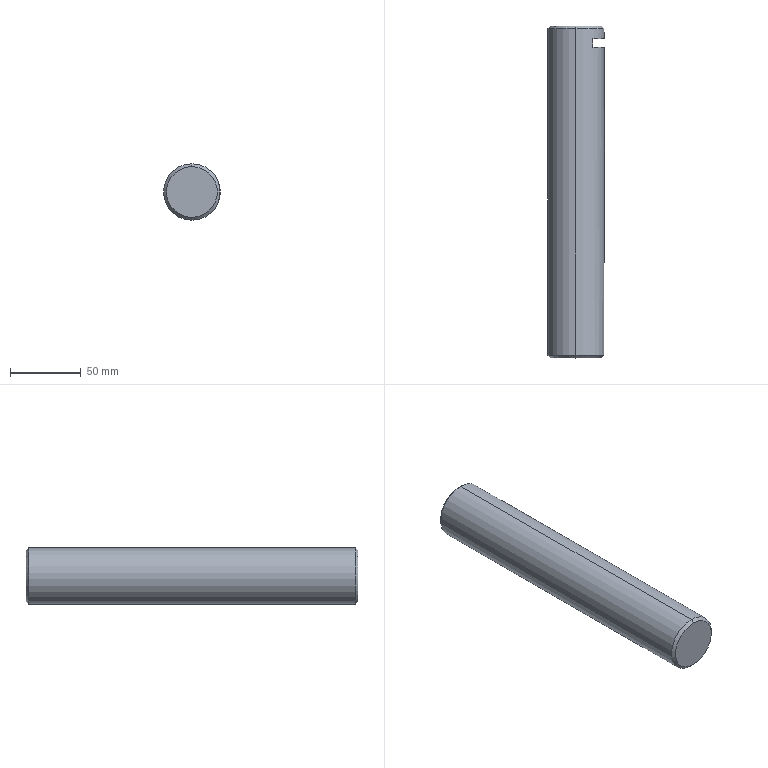Part | STEP file | 05-Sprocket shaft | 1 solid | 11 faces | box 40 x 235 x 40 mm | volume 293750 mm3 | plane 5 | cone 4 | cylinder 2 | commonest cylinder face diameters 40 x2
STEP:
#1=CARTESIAN_POINT('',(0.,0.,0.));
#2=DIRECTION('',(0.,0.,1.));
#3=DIRECTION('',(1.,0.,0.));
#4=AXIS2_PLACEMENT_3D('',#1,#2,#3);
#5=CARTESIAN_POINT('',(0.,235.,18.));
#6=VERTEX_POINT('',#5);
#7=CARTESIAN_POINT('',(0.,235.,-18.));
#8=VERTEX_POINT('',#7);
#9=CARTESIAN_POINT('',(0.,235.,0.));
#10=DIRECTION('',(0.,1.,0.));
#11=DIRECTION('',(0.,0.,1.));
#12=AXIS2_PLACEMENT_3D('',#9,#10,#11);
#13=CIRCLE('',#12,18.);
#14=CARTESIAN_POINT('',(0.,235.,0.));
#15=DIRECTION('',(0.,-1.,0.));
#16=DIRECTION('',(0.,0.,-1.));
#17=AXIS2_PLACEMENT_3D('',#14,#15,#16);
#18=CONICAL_SURFACE('',#17,18.,0.7854);
#19=CARTESIAN_POINT('',(3.142,0.));
#20=DIRECTION('',(-1.,0.));
#21=VECTOR('',#20,1.);
#22=LINE('',#19,#21);
#23=(GEOMETRIC_REPRESENTATION_CONTEXT(2)PARAMETRIC_REPRESENTATION_CONTEXT()REPRESENTATION_CONTEXT('',''));
#24=DEFINITIONAL_REPRESENTATION('',(#22),#23);
#25=PCURVE('',#18,#24);
#26=CARTESIAN_POINT('',(0.,235.,0.));
#27=DIRECTION('',(0.,1.,0.));
#28=DIRECTION('',(0.,0.,1.));
#29=AXIS2_PLACEMENT_3D('',#26,#27,#28);
#30=PLANE('',#29);
#31=CARTESIAN_POINT('',(0.,0.));
#32=DIRECTION('',(1.,0.));
#33=AXIS2_PLACEMENT_2D('',#31,#32);
#34=CIRCLE('',#33,18.);
#35=(GEOMETRIC_REPRESENTATION_CONTEXT(2)PARAMETRIC_REPRESENTATION_CONTEXT()REPRESENTATION_CONTEXT('',''));
#36=DEFINITIONAL_REPRESENTATION('',(#34),#35);
#37=PCURVE('',#30,#36);
#38=SURFACE_CURVE('',#13,(#25,#37),.PCURVE_S1.);
#39=EDGE_CURVE('',#6,#8,#38,.T.);
#40=ORIENTED_EDGE('',*,*,#39,.F.);
#41=CARTESIAN_POINT('',(0.,233.,20.));
#42=VERTEX_POINT('',#41);
#43=CARTESIAN_POINT('',(0.,235.,18.));
#44=DIRECTION('',(0.,-0.7071,0.7071));
#45=VECTOR('',#44,1.);
#46=LINE('',#43,#45);
#47=CARTESIAN_POINT('',(3.142,0.));
#48=DIRECTION('',(0.,1.));
#49=VECTOR('',#48,1.);
#50=LINE('',#47,#49);
#51=(GEOMETRIC_REPRESENTATION_CONTEXT(2)PARAMETRIC_REPRESENTATION_CONTEXT()REPRESENTATION_CONTEXT('',''));
#52=DEFINITIONAL_REPRESENTATION('',(#50),#51);
#53=PCURVE('',#18,#52);
#54=CARTESIAN_POINT('',(0.,235.,0.));
#55=DIRECTION('',(0.,-1.,0.));
#56=DIRECTION('',(0.,0.,-1.));
#57=AXIS2_PLACEMENT_3D('',#54,#55,#56);
#58=CONICAL_SURFACE('',#57,18.,0.7854);
#59=CARTESIAN_POINT('',(3.142,0.));
#60=DIRECTION('',(0.,1.));
#61=VECTOR('',#60,1.);
#62=LINE('',#59,#61);
#63=(GEOMETRIC_REPRESENTATION_CONTEXT(2)PARAMETRIC_REPRESENTATION_CONTEXT()REPRESENTATION_CONTEXT('',''));
#64=DEFINITIONAL_REPRESENTATION('',(#62),#63);
#65=PCURVE('',#58,#64);
#66=SURFACE_CURVE('',#46,(#53,#65),.PCURVE_S1.);
#67=EDGE_CURVE('',#6,#42,#66,.T.);
#68=ORIENTED_EDGE('',*,*,#67,.T.);
#69=CARTESIAN_POINT('',(0.,233.,-20.));
#70=VERTEX_POINT('',#69);
#71=CARTESIAN_POINT('',(0.,233.,0.));
#72=DIRECTION('',(0.,-1.,0.));
#73=DIRECTION('',(0.,0.,1.));
#74=AXIS2_PLACEMENT_3D('',#71,#72,#73);
#75=CIRCLE('',#74,20.);
#76=CARTESIAN_POINT('',(-3.142,2.));
#77=DIRECTION('',(1.,0.));
#78=VECTOR('',#77,1.);
#79=LINE('',#76,#78);
#80=(GEOMETRIC_REPRESENTATION_CONTEXT(2)PARAMETRIC_REPRESENTATION_CONTEXT()REPRESENTATION_CONTEXT('',''));
#81=DEFINITIONAL_REPRESENTATION('',(#79),#80);
#82=PCURVE('',#18,#81);
#83=CARTESIAN_POINT('',(0.,235.,0.));
#84=DIRECTION('',(0.,-1.,0.));
#85=DIRECTION('',(0.,0.,-1.));
#86=AXIS2_PLACEMENT_3D('',#83,#84,#85);
#87=CYLINDRICAL_SURFACE('',#86,20.);
#88=CARTESIAN_POINT('',(-3.142,2.));
#89=DIRECTION('',(1.,0.));
#90=VECTOR('',#89,1.);
#91=LINE('',#88,#90);
#92=(GEOMETRIC_REPRESENTATION_CONTEXT(2)PARAMETRIC_REPRESENTATION_CONTEXT()REPRESENTATION_CONTEXT('',''));
#93=DEFINITIONAL_REPRESENTATION('',(#91),#92);
#94=PCURVE('',#87,#93);
#95=SURFACE_CURVE('',#75,(#82,#94),.PCURVE_S1.);
#96=EDGE_CURVE('',#70,#42,#95,.T.);
#97=ORIENTED_EDGE('',*,*,#96,.F.);
#98=CARTESIAN_POINT('',(0.,235.,-18.));
#99=DIRECTION('',(0.,-0.7071,-0.7071));
#100=VECTOR('',#99,1.);
#101=LINE('',#98,#100);
#102=CARTESIAN_POINT('',(0.,0.));
#103=DIRECTION('',(0.,1.));
#104=VECTOR('',#103,1.);
#105=LINE('',#102,#104);
#106=(GEOMETRIC_REPRESENTATION_CONTEXT(2)PARAMETRIC_REPRESENTATION_CONTEXT()REPRESENTATION_CONTEXT('',''));
#107=DEFINITIONAL_REPRESENTATION('',(#105),#106);
#108=PCURVE('',#18,#107);
#109=CARTESIAN_POINT('',(6.283,0.));
#110=DIRECTION('',(0.,1.));
#111=VECTOR('',#110,1.);
#112=LINE('',#109,#111);
#113=(GEOMETRIC_REPRESENTATION_CONTEXT(2)PARAMETRIC_REPRESENTATION_CONTEXT()REPRESENTATION_CONTEXT('',''));
#114=DEFINITIONAL_REPRESENTATION('',(#112),#113);
#115=PCURVE('',#58,#114);
#116=SURFACE_CURVE('',#101,(#108,#115),.PCURVE_S1.);
#117=EDGE_CURVE('',#8,#70,#116,.T.);
#118=ORIENTED_EDGE('',*,*,#117,.F.);
#119=EDGE_LOOP('',(#40,#68,#97,#118));
#120=FACE_BOUND('',#119,.T.);
#121=ADVANCED_FACE('',(#120),#18,.T.);
#122=CARTESIAN_POINT('',(0.,0.,-18.));
#123=VERTEX_POINT('',#122);
#124=CARTESIAN_POINT('',(0.,0.,18.));
#125=VERTEX_POINT('',#124);
#126=CARTESIAN_POINT('',(0.,0.,0.));
#127=DIRECTION('',(0.,-1.,0.));
#128=DIRECTION('',(0.,0.,1.));
#129=AXIS2_PLACEMENT_3D('',#126,#127,#128);
#130=CIRCLE('',#129,18.);
#131=CARTESIAN_POINT('',(0.,2.,0.));
#132=DIRECTION('',(0.,1.,0.));
#133=DIRECTION('',(0.,0.,1.));
#134=AXIS2_PLACEMENT_3D('',#131,#132,#133);
#135=CONICAL_SURFACE('',#134,20.,0.7854);
#136=CARTESIAN_POINT('',(6.283,-2.));
#137=DIRECTION('',(-1.,0.));
#138=VECTOR('',#137,1.);
#139=LINE('',#136,#138);
#140=(GEOMETRIC_REPRESENTATION_CONTEXT(2)PARAMETRIC_REPRESENTATION_CONTEXT()REPRESENTATION_CONTEXT('',''));
#141=DEFINITIONAL_REPRESENTATION('',(#139),#140);
#142=PCURVE('',#135,#141);
#143=CARTESIAN_POINT('',(0.,0.,0.));
#144=DIRECTION('',(0.,1.,0.));
#145=DIRECTION('',(0.,0.,1.));
#146=AXIS2_PLACEMENT_3D('',#143,#144,#145);
#147=PLANE('',#146);
#148=CARTESIAN_POINT('',(18.,0.));
#149=CARTESIAN_POINT('',(18.,-31.177));
#150=CARTESIAN_POINT('',(-9.,-15.588));
#151=CARTESIAN_POINT('',(-36.,0.));
#152=CARTESIAN_POINT('',(-9.,15.588));
#153=CARTESIAN_POINT('',(18.,31.177));
#154=CARTESIAN_POINT('',(18.,0.));
#155=(BOUNDED_CURVE()B_SPLINE_CURVE(2,(#148,#149,#150,#151,#152,#153,#154),.UNSPECIFIED.,.T.,.F.)B_SPLINE_CURVE_WITH_KNOTS((1,2,2,2,2,1),(-2.094,0.,2.094,4.189,6.283,8.378),.UNSPECIFIED.)CURVE()GEOMETRIC_REPRESENTATION_ITEM()RATIONAL_B_SPLINE_CURVE((1.,0.5,1.,0.5,1.,0.5,1.))REPRESENTATION_ITEM(''));
#156=(GEOMETRIC_REPRESENTATION_CONTEXT(2)PARAMETRIC_REPRESENTATION_CONTEXT()REPRESENTATION_CONTEXT('',''));
#157=DEFINITIONAL_REPRESENTATION('',(#155),#156);
#158=PCURVE('',#147,#157);
#159=SURFACE_CURVE('',#130,(#142,#158),.PCURVE_S1.);
#160=EDGE_CURVE('',#123,#125,#159,.T.);
#161=ORIENTED_EDGE('',*,*,#160,.F.);
#162=CARTESIAN_POINT('',(0.,2.,-20.));
#163=VERTEX_POINT('',#162);
#164=CARTESIAN_POINT('',(0.,2.,-20.));
#165=DIRECTION('',(0.,0.7071,-0.7071));
#166=VECTOR('',#165,1.);
#167=LINE('',#164,#166);
#168=CARTESIAN_POINT('',(3.142,0.));
#169=DIRECTION('',(0.,1.));
#170=VECTOR('',#169,1.);
#171=LINE('',#168,#170);
#172=(GEOMETRIC_REPRESENTATION_CONTEXT(2)PARAMETRIC_REPRESENTATION_CONTEXT()REPRESENTATION_CONTEXT('',''));
#173=DEFINITIONAL_REPRESENTATION('',(#171),#172);
#174=PCURVE('',#135,#173);
#175=CARTESIAN_POINT('',(0.,2.,0.));
#176=DIRECTION('',(0.,1.,0.));
#177=DIRECTION('',(0.,0.,1.));
#178=AXIS2_PLACEMENT_3D('',#175,#176,#177);
#179=CONICAL_SURFACE('',#178,20.,0.7854);
#180=CARTESIAN_POINT('',(3.142,0.));
#181=DIRECTION('',(0.,1.));
#182=VECTOR('',#181,1.);
#183=LINE('',#180,#182);
#184=(GEOMETRIC_REPRESENTATION_CONTEXT(2)PARAMETRIC_REPRESENTATION_CONTEXT()REPRESENTATION_CONTEXT('',''));
#185=DEFINITIONAL_REPRESENTATION('',(#183),#184);
#186=PCURVE('',#179,#185);
#187=SURFACE_CURVE('',#167,(#174,#186),.PCURVE_S1.);
#188=EDGE_CURVE('',#123,#163,#187,.T.);
#189=ORIENTED_EDGE('',*,*,#188,.T.);
#190=CARTESIAN_POINT('',(0.,2.,20.));
#191=VERTEX_POINT('',#190);
#192=CARTESIAN_POINT('',(0.,2.,0.));
#193=DIRECTION('',(0.,1.,0.));
#194=DIRECTION('',(0.,0.,1.));
#195=AXIS2_PLACEMENT_3D('',#192,#193,#194);
#196=CIRCLE('',#195,20.);
#197=CARTESIAN_POINT('',(0.,0.));
#198=DIRECTION('',(1.,0.));
#199=VECTOR('',#198,1.);
#200=LINE('',#197,#199);
#201=(GEOMETRIC_REPRESENTATION_CONTEXT(2)PARAMETRIC_REPRESENTATION_CONTEXT()REPRESENTATION_CONTEXT('',''));
#202=DEFINITIONAL_REPRESENTATION('',(#200),#201);
#203=PCURVE('',#135,#202);
#204=CARTESIAN_POINT('',(3.142,233.));
#205=DIRECTION('',(-1.,0.));
#206=VECTOR('',#205,1.);
#207=LINE('',#204,#206);
#208=(GEOMETRIC_REPRESENTATION_CONTEXT(2)PARAMETRIC_REPRESENTATION_CONTEXT()REPRESENTATION_CONTEXT('',''));
#209=DEFINITIONAL_REPRESENTATION('',(#207),#208);
#210=PCURVE('',#87,#209);
#211=SURFACE_CURVE('',#196,(#203,#210),.PCURVE_S1.);
#212=EDGE_CURVE('',#191,#163,#211,.T.);
#213=ORIENTED_EDGE('',*,*,#212,.F.);
#214=CARTESIAN_POINT('',(0.,2.,20.));
#215=DIRECTION('',(0.,0.7071,0.7071));
#216=VECTOR('',#215,1.);
#217=LINE('',#214,#216);
#218=CARTESIAN_POINT('',(0.,0.));
#219=DIRECTION('',(0.,1.));
#220=VECTOR('',#219,1.);
#221=LINE('',#218,#220);
#222=(GEOMETRIC_REPRESENTATION_CONTEXT(2)PARAMETRIC_REPRESENTATION_CONTEXT()REPRESENTATION_CONTEXT('',''));
#223=DEFINITIONAL_REPRESENTATION('',(#221),#222);
#224=PCURVE('',#135,#223);
#225=CARTESIAN_POINT('',(6.283,0.));
#226=DIRECTION('',(0.,1.));
#227=VECTOR('',#226,1.);
#228=LINE('',#225,#227);
#229=(GEOMETRIC_REPRESENTATION_CONTEXT(2)PARAMETRIC_REPRESENTATION_CONTEXT()REPRESENTATION_CONTEXT('',''));
#230=DEFINITIONAL_REPRESENTATION('',(#228),#229);
#231=PCURVE('',#179,#230);
#232=SURFACE_CURVE('',#217,(#224,#231),.PCURVE_S1.);
#233=EDGE_CURVE('',#125,#191,#232,.T.);
#234=ORIENTED_EDGE('',*,*,#233,.F.);
#235=EDGE_LOOP('',(#161,#189,#213,#234));
#236=FACE_BOUND('',#235,.T.);
#237=ADVANCED_FACE('',(#236),#135,.T.);
#238=CARTESIAN_POINT('',(12.,226.,16.));
#239=VERTEX_POINT('',#238);
#240=CARTESIAN_POINT('',(12.,220.,16.));
#241=VERTEX_POINT('',#240);
#242=CARTESIAN_POINT('',(12.,235.,16.));
#243=DIRECTION('',(0.,-1.,0.));
#244=VECTOR('',#243,1.);
#245=LINE('',#242,#244);
#246=CARTESIAN_POINT('',(2.498,0.));
#247=DIRECTION('',(0.,1.));
#248=VECTOR('',#247,1.);
#249=LINE('',#246,#248);
#250=(GEOMETRIC_REPRESENTATION_CONTEXT(2)PARAMETRIC_REPRESENTATION_CONTEXT()REPRESENTATION_CONTEXT('',''));
#251=DEFINITIONAL_REPRESENTATION('',(#249),#250);
#252=PCURVE('',#87,#251);
#253=CARTESIAN_POINT('',(12.,0.,0.));
#254=DIRECTION('',(1.,0.,0.));
#255=DIRECTION('',(0.,0.,-1.));
#256=AXIS2_PLACEMENT_3D('',#253,#254,#255);
#257=PLANE('',#256);
#258=CARTESIAN_POINT('',(-16.,235.));
#259=DIRECTION('',(0.,-1.));
#260=VECTOR('',#259,1.);
#261=LINE('',#258,#260);
#262=(GEOMETRIC_REPRESENTATION_CONTEXT(2)PARAMETRIC_REPRESENTATION_CONTEXT()REPRESENTATION_CONTEXT('',''));
#263=DEFINITIONAL_REPRESENTATION('',(#261),#262);
#264=PCURVE('',#257,#263);
#265=SURFACE_CURVE('',#245,(#252,#264),.PCURVE_S1.);
#266=EDGE_CURVE('',#239,#241,#265,.T.);
#267=ORIENTED_EDGE('',*,*,#266,.F.);
#268=CARTESIAN_POINT('',(12.,226.,-16.));
#269=VERTEX_POINT('',#268);
#270=CARTESIAN_POINT('',(0.,226.,0.));
#271=DIRECTION('',(0.,-1.,0.));
#272=DIRECTION('',(0.,0.,-1.));
#273=AXIS2_PLACEMENT_3D('',#270,#271,#272);
#274=CIRCLE('',#273,20.);
#275=CARTESIAN_POINT('',(0.,9.));
#276=DIRECTION('',(1.,0.));
#277=VECTOR('',#276,1.);
#278=LINE('',#275,#277);
#279=(GEOMETRIC_REPRESENTATION_CONTEXT(2)PARAMETRIC_REPRESENTATION_CONTEXT()REPRESENTATION_CONTEXT('',''));
#280=DEFINITIONAL_REPRESENTATION('',(#278),#279);
#281=PCURVE('',#87,#280);
#282=CARTESIAN_POINT('',(247.,226.,35.835));
#283=DIRECTION('',(0.,-1.,0.));
#284=DIRECTION('',(0.,0.,-1.));
#285=AXIS2_PLACEMENT_3D('',#282,#283,#284);
#286=PLANE('',#285);
#287=CARTESIAN_POINT('',(35.835,-247.));
#288=DIRECTION('',(1.,0.));
#289=AXIS2_PLACEMENT_2D('',#287,#288);
#290=CIRCLE('',#289,20.);
#291=(GEOMETRIC_REPRESENTATION_CONTEXT(2)PARAMETRIC_REPRESENTATION_CONTEXT()REPRESENTATION_CONTEXT('',''));
#292=DEFINITIONAL_REPRESENTATION('',(#290),#291);
#293=PCURVE('',#286,#292);
#294=SURFACE_CURVE('',#274,(#281,#293),.PCURVE_S1.);
#295=EDGE_CURVE('',#269,#239,#294,.T.);
#296=ORIENTED_EDGE('',*,*,#295,.F.);
#297=CARTESIAN_POINT('',(12.,220.,-16.));
#298=VERTEX_POINT('',#297);
#299=CARTESIAN_POINT('',(12.,235.,-16.));
#300=DIRECTION('',(0.,1.,0.));
#301=VECTOR('',#300,1.);
#302=LINE('',#299,#301);
#303=CARTESIAN_POINT('',(0.6435,0.));
#304=DIRECTION('',(0.,-1.));
#305=VECTOR('',#304,1.);
#306=LINE('',#303,#305);
#307=(GEOMETRIC_REPRESENTATION_CONTEXT(2)PARAMETRIC_REPRESENTATION_CONTEXT()REPRESENTATION_CONTEXT('',''));
#308=DEFINITIONAL_REPRESENTATION('',(#306),#307);
#309=PCURVE('',#87,#308);
#310=CARTESIAN_POINT('',(16.,235.));
#311=DIRECTION('',(0.,1.));
#312=VECTOR('',#311,1.);
#313=LINE('',#310,#312);
#314=(GEOMETRIC_REPRESENTATION_CONTEXT(2)PARAMETRIC_REPRESENTATION_CONTEXT()REPRESENTATION_CONTEXT('',''));
#315=DEFINITIONAL_REPRESENTATION('',(#313),#314);
#316=PCURVE('',#257,#315);
#317=SURFACE_CURVE('',#302,(#309,#316),.PCURVE_S1.);
#318=EDGE_CURVE('',#298,#269,#317,.T.);
#319=ORIENTED_EDGE('',*,*,#318,.F.);
#320=CARTESIAN_POINT('',(0.,220.,0.));
#321=DIRECTION('',(0.,1.,0.));
#322=DIRECTION('',(0.,0.,1.));
#323=AXIS2_PLACEMENT_3D('',#320,#321,#322);
#324=CIRCLE('',#323,20.);
#325=CARTESIAN_POINT('',(3.142,15.));
#326=DIRECTION('',(-1.,0.));
#327=VECTOR('',#326,1.);
#328=LINE('',#325,#327);
#329=(GEOMETRIC_REPRESENTATION_CONTEXT(2)PARAMETRIC_REPRESENTATION_CONTEXT()REPRESENTATION_CONTEXT('',''));
#330=DEFINITIONAL_REPRESENTATION('',(#328),#329);
#331=PCURVE('',#87,#330);
#332=CARTESIAN_POINT('',(247.,220.,35.835));
#333=DIRECTION('',(0.,1.,0.));
#334=DIRECTION('',(0.,0.,1.));
#335=AXIS2_PLACEMENT_3D('',#332,#333,#334);
#336=PLANE('',#335);
#337=CARTESIAN_POINT('',(-35.835,-247.));
#338=DIRECTION('',(1.,0.));
#339=AXIS2_PLACEMENT_2D('',#337,#338);
#340=CIRCLE('',#339,20.);
#341=(GEOMETRIC_REPRESENTATION_CONTEXT(2)PARAMETRIC_REPRESENTATION_CONTEXT()REPRESENTATION_CONTEXT('',''));
#342=DEFINITIONAL_REPRESENTATION('',(#340),#341);
#343=PCURVE('',#336,#342);
#344=SURFACE_CURVE('',#324,(#331,#343),.PCURVE_S1.);
#345=EDGE_CURVE('',#241,#298,#344,.T.);
#346=ORIENTED_EDGE('',*,*,#345,.F.);
#347=EDGE_LOOP('',(#267,#296,#319,#346));
#348=FACE_BOUND('',#347,.T.);
#349=ORIENTED_EDGE('',*,*,#96,.T.);
#350=CARTESIAN_POINT('',(0.,235.,20.));
#351=DIRECTION('',(0.,-1.,0.));
#352=VECTOR('',#351,1.);
#353=LINE('',#350,#352);
#354=CARTESIAN_POINT('',(3.142,0.));
#355=DIRECTION('',(0.,1.));
#356=VECTOR('',#355,1.);
#357=LINE('',#354,#356);
#358=(GEOMETRIC_REPRESENTATION_CONTEXT(2)PARAMETRIC_REPRESENTATION_CONTEXT()REPRESENTATION_CONTEXT('',''));
#359=DEFINITIONAL_REPRESENTATION('',(#357),#358);
#360=PCURVE('',#87,#359);
#361=CARTESIAN_POINT('',(0.,235.,0.));
#362=DIRECTION('',(0.,-1.,0.));
#363=DIRECTION('',(0.,0.,-1.));
#364=AXIS2_PLACEMENT_3D('',#361,#362,#363);
#365=CYLINDRICAL_SURFACE('',#364,20.);
#366=CARTESIAN_POINT('',(3.142,0.));
#367=DIRECTION('',(0.,1.));
#368=VECTOR('',#367,1.);
#369=LINE('',#366,#368);
#370=(GEOMETRIC_REPRESENTATION_CONTEXT(2)PARAMETRIC_REPRESENTATION_CONTEXT()REPRESENTATION_CONTEXT('',''));
#371=DEFINITIONAL_REPRESENTATION('',(#369),#370);
#372=PCURVE('',#365,#371);
#373=SURFACE_CURVE('',#353,(#360,#372),.PCURVE_S1.);
#374=EDGE_CURVE('',#42,#191,#373,.T.);
#375=ORIENTED_EDGE('',*,*,#374,.T.);
#376=ORIENTED_EDGE('',*,*,#212,.T.);
#377=CARTESIAN_POINT('',(0.,235.,-20.));
#378=DIRECTION('',(0.,-1.,0.));
#379=VECTOR('',#378,1.);
#380=LINE('',#377,#379);
#381=CARTESIAN_POINT('',(0.,0.));
#382=DIRECTION('',(0.,1.));
#383=VECTOR('',#382,1.);
#384=LINE('',#381,#383);
#385=(GEOMETRIC_REPRESENTATION_CONTEXT(2)PARAMETRIC_REPRESENTATION_CONTEXT()REPRESENTATION_CONTEXT('',''));
#386=DEFINITIONAL_REPRESENTATION('',(#384),#385);
#387=PCURVE('',#87,#386);
#388=CARTESIAN_POINT('',(6.283,0.));
#389=DIRECTION('',(0.,1.));
#390=VECTOR('',#389,1.);
#391=LINE('',#388,#390);
#392=(GEOMETRIC_REPRESENTATION_CONTEXT(2)PARAMETRIC_REPRESENTATION_CONTEXT()REPRESENTATION_CONTEXT('',''));
#393=DEFINITIONAL_REPRESENTATION('',(#391),#392);
#394=PCURVE('',#365,#393);
#395=SURFACE_CURVE('',#380,(#387,#394),.PCURVE_S1.);
#396=EDGE_CURVE('',#70,#163,#395,.T.);
#397=ORIENTED_EDGE('',*,*,#396,.F.);
#398=EDGE_LOOP('',(#349,#375,#376,#397));
#399=FACE_BOUND('',#398,.T.);
#400=ADVANCED_FACE('',(#348,#399),#87,.T.);
#401=ORIENTED_EDGE('',*,*,#374,.F.);
#402=CARTESIAN_POINT('',(0.,233.,0.));
#403=DIRECTION('',(0.,-1.,0.));
#404=DIRECTION('',(0.,0.,1.));
#405=AXIS2_PLACEMENT_3D('',#402,#403,#404);
#406=CIRCLE('',#405,20.);
#407=CARTESIAN_POINT('',(3.142,2.));
#408=DIRECTION('',(1.,0.));
#409=VECTOR('',#408,1.);
#410=LINE('',#407,#409);
#411=(GEOMETRIC_REPRESENTATION_CONTEXT(2)PARAMETRIC_REPRESENTATION_CONTEXT()REPRESENTATION_CONTEXT('',''));
#412=DEFINITIONAL_REPRESENTATION('',(#410),#411);
#413=PCURVE('',#365,#412);
#414=CARTESIAN_POINT('',(3.142,2.));
#415=DIRECTION('',(1.,0.));
#416=VECTOR('',#415,1.);
#417=LINE('',#414,#416);
#418=(GEOMETRIC_REPRESENTATION_CONTEXT(2)PARAMETRIC_REPRESENTATION_CONTEXT()REPRESENTATION_CONTEXT('',''));
#419=DEFINITIONAL_REPRESENTATION('',(#417),#418);
#420=PCURVE('',#58,#419);
#421=SURFACE_CURVE('',#406,(#413,#420),.PCURVE_S1.);
#422=EDGE_CURVE('',#42,#70,#421,.T.);
#423=ORIENTED_EDGE('',*,*,#422,.T.);
#424=ORIENTED_EDGE('',*,*,#396,.T.);
#425=CARTESIAN_POINT('',(0.,2.,0.));
#426=DIRECTION('',(0.,1.,0.));
#427=DIRECTION('',(0.,0.,1.));
#428=AXIS2_PLACEMENT_3D('',#425,#426,#427);
#429=CIRCLE('',#428,20.);
#430=CARTESIAN_POINT('',(9.425,233.));
#431=DIRECTION('',(-1.,0.));
#432=VECTOR('',#431,1.);
#433=LINE('',#430,#432);
#434=(GEOMETRIC_REPRESENTATION_CONTEXT(2)PARAMETRIC_REPRESENTATION_CONTEXT()REPRESENTATION_CONTEXT('',''));
#435=DEFINITIONAL_REPRESENTATION('',(#433),#434);
#436=PCURVE('',#365,#435);
#437=CARTESIAN_POINT('',(0.,0.));
#438=DIRECTION('',(1.,0.));
#439=VECTOR('',#438,1.);
#440=LINE('',#437,#439);
#441=(GEOMETRIC_REPRESENTATION_CONTEXT(2)PARAMETRIC_REPRESENTATION_CONTEXT()REPRESENTATION_CONTEXT('',''));
#442=DEFINITIONAL_REPRESENTATION('',(#440),#441);
#443=PCURVE('',#179,#442);
#444=SURFACE_CURVE('',#429,(#436,#443),.PCURVE_S1.);
#445=EDGE_CURVE('',#163,#191,#444,.T.);
#446=ORIENTED_EDGE('',*,*,#445,.T.);
#447=EDGE_LOOP('',(#401,#423,#424,#446));
#448=FACE_BOUND('',#447,.T.);
#449=ADVANCED_FACE('',(#448),#365,.T.);
#450=CARTESIAN_POINT('',(0.,235.,0.));
#451=DIRECTION('',(0.,1.,0.));
#452=DIRECTION('',(0.,0.,1.));
#453=AXIS2_PLACEMENT_3D('',#450,#451,#452);
#454=CIRCLE('',#453,18.);
#455=CARTESIAN_POINT('',(0.,0.));
#456=DIRECTION('',(1.,0.));
#457=AXIS2_PLACEMENT_2D('',#455,#456);
#458=CIRCLE('',#457,18.);
#459=(GEOMETRIC_REPRESENTATION_CONTEXT(2)PARAMETRIC_REPRESENTATION_CONTEXT()REPRESENTATION_CONTEXT('',''));
#460=DEFINITIONAL_REPRESENTATION('',(#458),#459);
#461=PCURVE('',#30,#460);
#462=CARTESIAN_POINT('',(9.425,0.));
#463=DIRECTION('',(-1.,0.));
#464=VECTOR('',#463,1.);
#465=LINE('',#462,#464);
#466=(GEOMETRIC_REPRESENTATION_CONTEXT(2)PARAMETRIC_REPRESENTATION_CONTEXT()REPRESENTATION_CONTEXT('',''));
#467=DEFINITIONAL_REPRESENTATION('',(#465),#466);
#468=PCURVE('',#58,#467);
#469=SURFACE_CURVE('',#454,(#461,#468),.PCURVE_S1.);
#470=EDGE_CURVE('',#8,#6,#469,.T.);
#471=ORIENTED_EDGE('',*,*,#470,.T.);
#472=ORIENTED_EDGE('',*,*,#39,.T.);
#473=EDGE_LOOP('',(#471,#472));
#474=FACE_BOUND('',#473,.T.);
#475=ADVANCED_FACE('',(#474),#30,.T.);
#476=CARTESIAN_POINT('',(0.,0.,0.));
#477=DIRECTION('',(0.,-1.,0.));
#478=DIRECTION('',(0.,0.,1.));
#479=AXIS2_PLACEMENT_3D('',#476,#477,#478);
#480=CIRCLE('',#479,18.);
#481=CARTESIAN_POINT('',(18.,0.));
#482=CARTESIAN_POINT('',(18.,-31.177));
#483=CARTESIAN_POINT('',(-9.,-15.588));
#484=CARTESIAN_POINT('',(-36.,0.));
#485=CARTESIAN_POINT('',(-9.,15.588));
#486=CARTESIAN_POINT('',(18.,31.177));
#487=CARTESIAN_POINT('',(18.,0.));
#488=(BOUNDED_CURVE()B_SPLINE_CURVE(2,(#481,#482,#483,#484,#485,#486,#487),.UNSPECIFIED.,.T.,.F.)B_SPLINE_CURVE_WITH_KNOTS((1,2,2,2,2,1),(-2.094,0.,2.094,4.189,6.283,8.378),.UNSPECIFIED.)CURVE()GEOMETRIC_REPRESENTATION_ITEM()RATIONAL_B_SPLINE_CURVE((1.,0.5,1.,0.5,1.,0.5,1.))REPRESENTATION_ITEM(''));
#489=(GEOMETRIC_REPRESENTATION_CONTEXT(2)PARAMETRIC_REPRESENTATION_CONTEXT()REPRESENTATION_CONTEXT('',''));
#490=DEFINITIONAL_REPRESENTATION('',(#488),#489);
#491=PCURVE('',#147,#490);
#492=CARTESIAN_POINT('',(6.283,-2.));
#493=DIRECTION('',(-1.,0.));
#494=VECTOR('',#493,1.);
#495=LINE('',#492,#494);
#496=(GEOMETRIC_REPRESENTATION_CONTEXT(2)PARAMETRIC_REPRESENTATION_CONTEXT()REPRESENTATION_CONTEXT('',''));
#497=DEFINITIONAL_REPRESENTATION('',(#495),#496);
#498=PCURVE('',#179,#497);
#499=SURFACE_CURVE('',#480,(#491,#498),.PCURVE_S1.);
#500=EDGE_CURVE('',#125,#123,#499,.T.);
#501=ORIENTED_EDGE('',*,*,#500,.T.);
#502=ORIENTED_EDGE('',*,*,#160,.T.);
#503=EDGE_LOOP('',(#501,#502));
#504=FACE_BOUND('',#503,.T.);
#505=ADVANCED_FACE('',(#504),#147,.F.);
#506=ORIENTED_EDGE('',*,*,#345,.T.);
#507=CARTESIAN_POINT('',(12.,220.,35.835));
#508=DIRECTION('',(0.,0.,-1.));
#509=VECTOR('',#508,1.);
#510=LINE('',#507,#509);
#511=CARTESIAN_POINT('',(0.,-235.));
#512=DIRECTION('',(-1.,0.));
#513=VECTOR('',#512,1.);
#514=LINE('',#511,#513);
#515=(GEOMETRIC_REPRESENTATION_CONTEXT(2)PARAMETRIC_REPRESENTATION_CONTEXT()REPRESENTATION_CONTEXT('',''));
#516=DEFINITIONAL_REPRESENTATION('',(#514),#515);
#517=PCURVE('',#336,#516);
#518=CARTESIAN_POINT('',(-35.835,220.));
#519=DIRECTION('',(1.,0.));
#520=VECTOR('',#519,1.);
#521=LINE('',#518,#520);
#522=(GEOMETRIC_REPRESENTATION_CONTEXT(2)PARAMETRIC_REPRESENTATION_CONTEXT()REPRESENTATION_CONTEXT('',''));
#523=DEFINITIONAL_REPRESENTATION('',(#521),#522);
#524=PCURVE('',#257,#523);
#525=SURFACE_CURVE('',#510,(#517,#524),.PCURVE_S1.);
#526=EDGE_CURVE('',#241,#298,#525,.T.);
#527=ORIENTED_EDGE('',*,*,#526,.F.);
#528=EDGE_LOOP('',(#506,#527));
#529=FACE_BOUND('',#528,.T.);
#530=ADVANCED_FACE('',(#529),#336,.T.);
#531=ORIENTED_EDGE('',*,*,#295,.T.);
#532=CARTESIAN_POINT('',(12.,226.,35.835));
#533=DIRECTION('',(0.,0.,1.));
#534=VECTOR('',#533,1.);
#535=LINE('',#532,#534);
#536=CARTESIAN_POINT('',(0.,-235.));
#537=DIRECTION('',(-1.,0.));
#538=VECTOR('',#537,1.);
#539=LINE('',#536,#538);
#540=(GEOMETRIC_REPRESENTATION_CONTEXT(2)PARAMETRIC_REPRESENTATION_CONTEXT()REPRESENTATION_CONTEXT('',''));
#541=DEFINITIONAL_REPRESENTATION('',(#539),#540);
#542=PCURVE('',#286,#541);
#543=CARTESIAN_POINT('',(-35.835,226.));
#544=DIRECTION('',(-1.,0.));
#545=VECTOR('',#544,1.);
#546=LINE('',#543,#545);
#547=(GEOMETRIC_REPRESENTATION_CONTEXT(2)PARAMETRIC_REPRESENTATION_CONTEXT()REPRESENTATION_CONTEXT('',''));
#548=DEFINITIONAL_REPRESENTATION('',(#546),#547);
#549=PCURVE('',#257,#548);
#550=SURFACE_CURVE('',#535,(#542,#549),.PCURVE_S1.);
#551=EDGE_CURVE('',#269,#239,#550,.T.);
#552=ORIENTED_EDGE('',*,*,#551,.F.);
#553=EDGE_LOOP('',(#531,#552));
#554=FACE_BOUND('',#553,.T.);
#555=ADVANCED_FACE('',(#554),#286,.T.);
#556=ORIENTED_EDGE('',*,*,#266,.T.);
#557=ORIENTED_EDGE('',*,*,#526,.T.);
#558=ORIENTED_EDGE('',*,*,#318,.T.);
#559=ORIENTED_EDGE('',*,*,#551,.T.);
#560=EDGE_LOOP('',(#556,#557,#558,#559));
#561=FACE_BOUND('',#560,.T.);
#562=ADVANCED_FACE('',(#561),#257,.T.);
#563=ORIENTED_EDGE('',*,*,#188,.F.);
#564=ORIENTED_EDGE('',*,*,#500,.F.);
#565=ORIENTED_EDGE('',*,*,#233,.T.);
#566=ORIENTED_EDGE('',*,*,#445,.F.);
#567=EDGE_LOOP('',(#563,#564,#565,#566));
#568=FACE_BOUND('',#567,.T.);
#569=ADVANCED_FACE('',(#568),#179,.T.);
#570=ORIENTED_EDGE('',*,*,#67,.F.);
#571=ORIENTED_EDGE('',*,*,#470,.F.);
#572=ORIENTED_EDGE('',*,*,#117,.T.);
#573=ORIENTED_EDGE('',*,*,#422,.F.);
#574=EDGE_LOOP('',(#570,#571,#572,#573));
#575=FACE_BOUND('',#574,.T.);
#576=ADVANCED_FACE('',(#575),#58,.T.);
#577=CLOSED_SHELL('',(#121,#237,#400,#449,#475,#505,#530,#555,#562,#569,#576));
#578=MANIFOLD_SOLID_BREP('',#577);
#579=(LENGTH_UNIT()NAMED_UNIT(*)SI_UNIT(.MILLI.,.METRE.));
#580=UNCERTAINTY_MEASURE_WITH_UNIT(LENGTH_MEASURE(0.0000001),#579,'','');
#581=(NAMED_UNIT(*)PLANE_ANGLE_UNIT()SI_UNIT($,.RADIAN.));
#582=(NAMED_UNIT(*)SI_UNIT($,.STERADIAN.)SOLID_ANGLE_UNIT());
#583=(GEOMETRIC_REPRESENTATION_CONTEXT(3)GLOBAL_UNCERTAINTY_ASSIGNED_CONTEXT((#580))GLOBAL_UNIT_ASSIGNED_CONTEXT((#579,#581,#582))REPRESENTATION_CONTEXT('',''));
#584=ADVANCED_BREP_SHAPE_REPRESENTATION('',(#4,#578),#583);